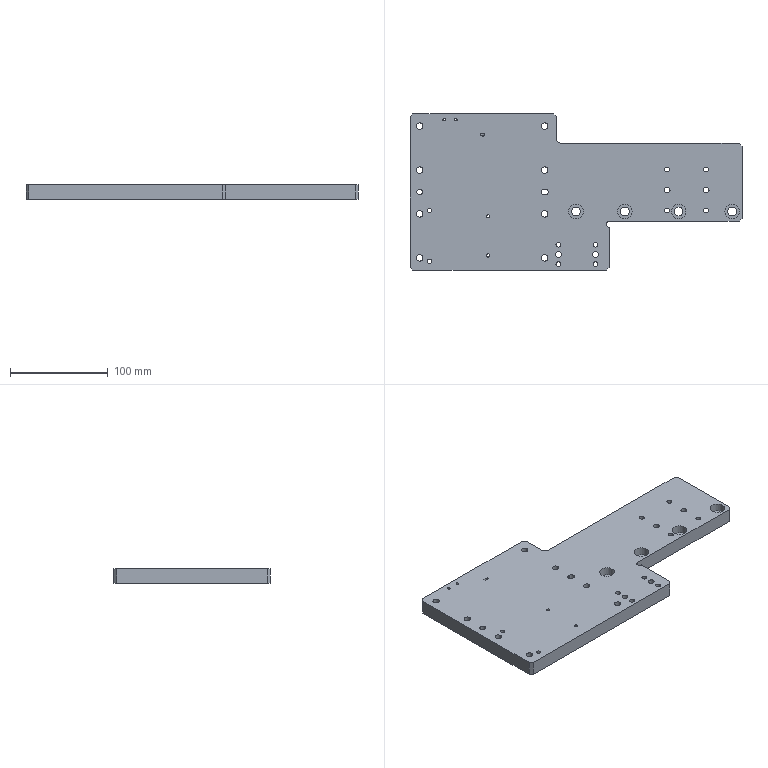CAM job | NX | 3-axis milling, drilling | part box 340 x 160 x 15 mm | stock box 345 x 165 x 15 mm
Tools:
number,name,description,diameter,corner_radius,flute_length,length,flutes
4,D4,平底铣刀-粗,4.0,0.0,25.0,75.0,2
6,D6,平底铣刀-粗,6.0,0.0,25.0,75.0,2
9,D10,平底铣刀-粗,10.0,0.0,35.0,75.0,2
11,D4-J,平底铣刀-精,4.0,0.0,50.0,75.0,2
7,D6-J,平底铣刀-精,6.0,0.0,25.0,75.0,2
2,D6倒角刀,倒角刀,6.0,0.0,3.0,25.0,2
20,M3X0.5,丝锥,2.5,0.0,35.0,50.0,2
21,M4X0.7,丝锥,3.3,0.0,35.0,50.0,2
22,M5X0.8,丝锥,4.2,0.0,35.0,50.0,2
23,M6X1.0,丝锥,5.0,0.0,35.0,50.0,2
19,D6铰刀,Drilling Tool,6.0,0.0,75.0,100.0,6
12,ZT2.6,钻头,2.6,0.0,35.0,50.0,2
13,ZT3.4,钻头,3.4,0.0,35.0,50.0,2
15,ZT5.1,钻头,5.1,0.0,35.0,50.0,2
18,ZT9,钻头,9.0,0.0,35.0,50.0,2
17,钻头6.6,Drilling Tool,6.6,0.0,35.0,50.0,2
17,ZT5.9,Drilling Tool,5.9,0.0,35.0,50.0,2
14,ZT4.3,Drilling Tool,4.3,0.0,50.0,75.0,4
Operations:
program,operation,operation_type,tool,method,geometry_group,spindle_rpm,surface_speed,feed_per_tooth,feed_cut,feed_plunge,cut_length_mm,path_length_mm,cut_time_min,machine_time_min
B,打点-深0.8,Operation,D6倒角刀,NONE,W-B,8000.0,150.796,0.0312,500.0,90.0,55.8,1148.348,0.1116,0.2209
B,通孔-M3螺纹底孔,Operation,ZT2.6,NONE,W-B,3000.0,23.562,0.05,300.0,90.0,44.0,201.042,0.1467,0.1624
B,通孔-M4螺纹底孔,Operation,ZT3.4,NONE,W-B,3000.0,31.102,0.05,300.0,90.0,44.0,229.012,0.1467,0.1652
B,通孔-M5螺纹底孔,Operation,ZT4.3,NONE,W-B,3000.0,39.584,0.0583,350.0,90.0,46.0,245.01,0.1314,0.1513
B,通孔-M6螺纹底孔,Operation,ZT5.1,NONE,W-B,2800.0,43.982,0.0625,350.0,90.0,184.0,756.311,0.5257,0.5829
B,通孔-精孔6.0预钻,Operation,ZT5.9,NONE,W-B,2500.0,46.339,0.05,250.0,90.0,103.516,643.438,0.4141,0.4681
B,通孔-8-10,Operation,ZT9,NONE,W-B,1800.0,50.894,0.0417,150.0,90.0,48.416,359.859,0.3228,0.3539
B,铣孔开粗D6_1,CylinderMilling,D6,NONE,W-B,8000.0,150.796,0.075,1200.0,100.0,1846.663,3136.863,1.539,1.668
B,铣孔精光D6_1,CylinderMilling,D6-J,精光步距切深关,W-B,8000.0,150.796,0.0312,500.0,100.0,356.922,1651.122,0.7138,0.8433
B,NG_钻倒角_4,Operation,D6倒角刀,METHOD,W-B,8000.0,150.796,0.0312,500.0,0.0,9.5,134.369,0.019,0.0315
B,NG_钻倒角_5,Operation,D6倒角刀,METHOD,W-B,8000.0,150.796,0.0312,500.0,0.0,10.4,163.912,0.0208,0.0362
B,铣倒角_5,PlanarMilling,D6倒角刀,METHOD,W-B,8000.0,150.796,0.0312,500.0,100.0,36.041,291.428,0.0721,0.0976
B,铣倒角_6,PlanarMilling,D6倒角刀,METHOD,W-B,8000.0,150.796,0.0312,500.0,100.0,159.505,1251.775,0.319,0.4282
B,铣倒角_7,PlanarMilling,D6倒角刀,METHOD,W-B,8000.0,150.796,0.0312,500.0,100.0,104.819,942.377,0.2096,0.2934
B,铣倒角_8,PlanarMilling,D6倒角刀,METHOD,W-B,8000.0,150.796,0.05,800.0,100.0,139.642,704.465,0.1746,0.231
B,铣倒角_9,PlanarMilling,D6倒角刀,NONE,W-B,8000.0,150.796,0.05,800.0,100.0,347.141,1523.096,0.4339,0.5515
B,C0.3封闭铣廓倒角6X45L_COPY,PlanarMilling,D6倒角刀,爬面_倒角-切深0-步距G,W-B,7000.0,131.0,0.1071,1500.0,100.0,29.685,125.685,0.0198,0.0294
B,REAMING,Operation,D6铰刀,METHOD,W-B,500.0,9.425,0.0167,50.0,0.0,85.0,606.407,1.7,1.752
B,通孔-攻牙M3,Operation,M3X0.5,METHOD,W-B,800.0,6.283,0.0003,0.5,90.0,38.0,189.042,76.0,76.015
B,通孔-攻牙M4,Operation,M4X0.7,METHOD,W-B,600.0,6.22,0.0006,0.7,90.0,38.0,217.012,54.286,54.304
B,通孔-攻牙M5,Operation,M5X0.8,METHOD,W-B,500.0,6.597,0.0008,0.8,90.0,39.0,231.01,48.75,48.769
B,通孔-攻牙M6,Operation,M6X1.0,METHOD,W-B,500.0,7.854,0.001,1.0,90.0,156.0,700.311,156.0,156.054
A,NG_打点-深2.1,Operation,D6倒角刀,NONE,W-A,3500.0,87.965,0.0357,500.0,90.0,62.0,1027.246,0.124,0.2205
A,NG_打点-深1.6,Operation,D6倒角刀,NONE,W-A,3500.0,87.965,0.0357,500.0,90.0,5.0,123.042,0.01,0.0218
A,打点-深1.6_COPY,Operation,D6倒角刀,NONE,W-A,3500.0,87.965,0.0357,500.0,90.0,20.0,476.407,0.04,0.0856
A,沉头孔打点-深1.5,Operation,D6倒角刀,NONE,W-A,3500.0,87.965,0.0357,500.0,90.0,10.0,283.028,0.02,0.0473
A,通孔-6-8,Operation,钻头6.6,NONE,W-A,1500.0,31.102,0.1333,400.0,90.0,100.042,705.155,0.2501,0.3106
A,通腰槽粗_1,VolumeBased25DMillingOperation,D4,METHOD,W-A,6000.0,75.0,0.0417,500.0,100.0,830.421,943.721,1.661,1.672
A,铣沉头_1,CylinderMilling,D6,METHOD,W-A,8000.0,150.796,0.1562,2500.0,100.0,2149.144,2742.344,0.8597,0.919
A,铣孔_1,CylinderMilling,D6-J,METHOD,W-A,8000.0,150.796,0.05,800.0,100.0,305.678,934.478,0.3821,0.445
A,外形粗_2,VolumeBased25DMillingOperation,D10,METHOD,W-A,6000.0,188.0,0.25,4000.0,80.0,31534.92,31647.92,7.884,7.895
A,外形D4清角,ZLevelMilling,D4-J,METHOD,W-A,6000.0,75.0,0.25,2500.0,80.0,823.875,937.771,0.3297,0.341
A,CHAMFER_2,SurfaceContour,D6倒角刀,METHOD,W-A,6000.0,113.0,0.125,1200.0,100.0,1222.473,2078.358,1.019,1.104
A,打点,Operation,D6倒角刀,METHOD,W-A,8000.0,150.796,0.1562,2500.0,0.0,10.0,201.063,0.004,0.0231
A,NG_钻倒角_1,Operation,D6倒角刀,METHOD,W-A,8000.0,150.796,0.0625,1000.0,0.0,9.5,134.369,0.0095,0.022
A,NG_钻倒角_2,Operation,D6倒角刀,METHOD,W-A,8000.0,150.796,0.0625,1000.0,0.0,10.4,163.912,0.0104,0.0258
A,NG_钻倒角_3,Operation,D6倒角刀,METHOD,W-A,8000.0,150.796,0.0625,1000.0,0.0,11.4,177.887,0.0114,0.028
A,铣倒角_1,PlanarMilling,D6倒角刀,METHOD,W-A,8000.0,150.796,0.0375,600.0,100.0,75.821,606.836,0.1264,0.1795
A,铣倒角_2,PlanarMilling,D6倒角刀,METHOD,W-A,8000.0,150.796,0.0375,600.0,100.0,94.776,935.176,0.158,0.242
A,铣倒角_3,PlanarMilling,D6倒角刀,METHOD,W-A,8000.0,150.796,0.075,1200.0,100.0,163.568,1375.986,0.1363,0.2575
A,铣倒角_4,PlanarMilling,D6倒角刀,METHOD,W-A,8000.0,150.796,0.0375,600.0,100.0,75.821,561.061,0.1264,0.1749
A,腰槽精_1,VolumeBased25DMillingOperation,D4-J,METHOD,W-A,6000.0,113.0,0.0167,200.0,100.0,31.798,181.932,0.159,0.174
A,外形半精_2,VolumeBased25DMillingOperation,D6-J,METHOD,W-A,6000.0,113.0,0.0833,1000.0,100.0,2029.001,2273.021,2.029,2.053
A,外形精_2,VolumeBased25DMillingOperation,D6-J,METHOD,W-A,6000.0,113.0,0.0833,1000.0,100.0,1014.3,1142.9,1.014,1.027